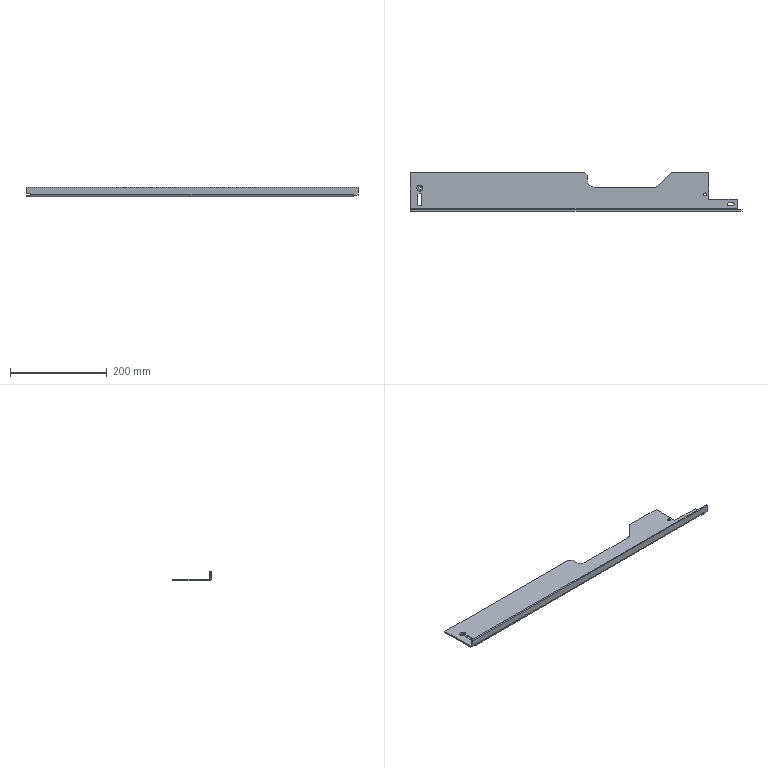Part | STEP file | Left guide rail PN_0060 | 1 solid | 42 faces | box 686 x 80 x 19 mm | volume 166808 mm3 | plane 29 | cylinder 11 | cone 2 | commonest cylinder face diameters 7 x3 6 x2 6.8 x2 4.2 x1 10.2 x1 20 x1